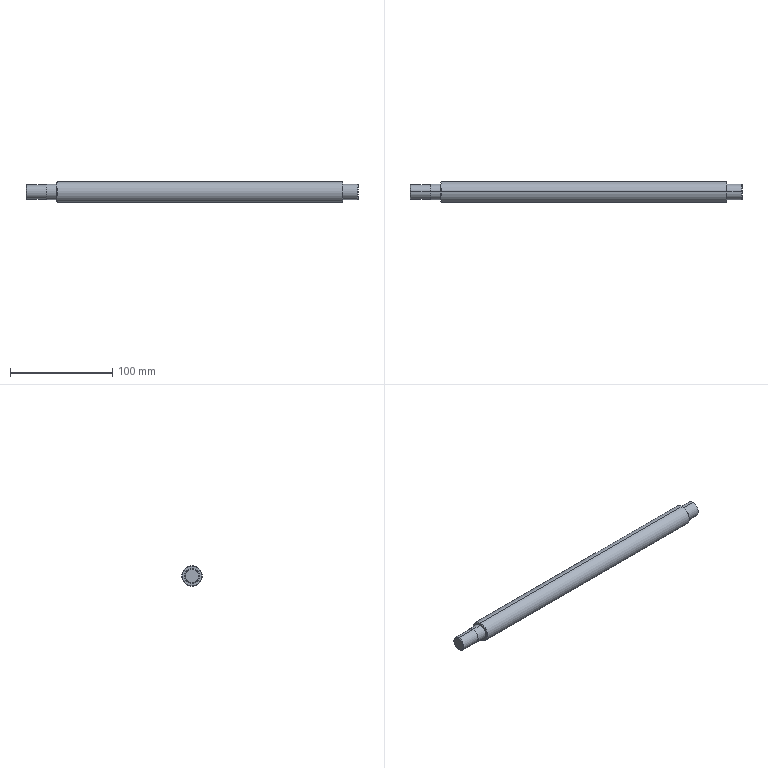Part | SolidWorks | features BaseBody 1 | 1 solid | 21 faces | box 325 x 20 x 20 mm | volume 95435 mm3 | cone 8 | cylinder 8 | plane 5 | commonest cylinder face diameters 15 x4 14 x2 20 x2
STEP:
#1=CARTESIAN_POINT('',(162.5,0.,7.));
#2=VERTEX_POINT('',#1);
#3=CARTESIAN_POINT('',(162.5,0.,-7.));
#4=VERTEX_POINT('',#3);
#5=CARTESIAN_POINT('',(162.5,0.,0.));
#6=DIRECTION('',(-1.,0.,0.));
#7=DIRECTION('',(0.,0.,1.));
#8=AXIS2_PLACEMENT_3D('',#5,#6,#7);
#9=CIRCLE('',#8,7.);
#10=EDGE_CURVE('',#2,#4,#9,.T.);
#11=ORIENTED_EDGE('',*,*,#10,.T.);
#12=CARTESIAN_POINT('',(162.,0.,-7.5));
#13=VERTEX_POINT('',#12);
#14=CARTESIAN_POINT('',(162.5,0.,-7.));
#15=DIRECTION('',(-0.7071,0.,-0.7071));
#16=VECTOR('',#15,1000.);
#17=LINE('',#14,#16);
#18=EDGE_CURVE('',#4,#13,#17,.T.);
#19=ORIENTED_EDGE('',*,*,#18,.T.);
#20=CARTESIAN_POINT('',(162.,0.,7.5));
#21=VERTEX_POINT('',#20);
#22=CARTESIAN_POINT('',(162.,0.,0.));
#23=DIRECTION('',(-1.,0.,0.));
#24=DIRECTION('',(0.,0.,1.));
#25=AXIS2_PLACEMENT_3D('',#22,#23,#24);
#26=CIRCLE('',#25,7.5);
#27=EDGE_CURVE('',#21,#13,#26,.T.);
#28=ORIENTED_EDGE('',*,*,#27,.F.);
#29=CARTESIAN_POINT('',(162.5,0.,7.));
#30=DIRECTION('',(-0.7071,0.,0.7071));
#31=VECTOR('',#30,1000.);
#32=LINE('',#29,#31);
#33=EDGE_CURVE('',#2,#21,#32,.T.);
#34=ORIENTED_EDGE('',*,*,#33,.F.);
#35=EDGE_LOOP('',(#11,#19,#28,#34));
#36=FACE_OUTER_BOUND('',#35,.T.);
#37=CARTESIAN_POINT('',(162.5,0.,0.));
#38=DIRECTION('',(-1.,0.,0.));
#39=DIRECTION('',(0.,0.,1.));
#40=AXIS2_PLACEMENT_3D('',#37,#38,#39);
#41=CONICAL_SURFACE('',#40,7.,0.7854);
#42=ADVANCED_FACE('',(#36),#41,.T.);
#43=ORIENTED_EDGE('',*,*,#27,.T.);
#44=CARTESIAN_POINT('',(147.5,0.,-7.5));
#45=VERTEX_POINT('',#44);
#46=CARTESIAN_POINT('',(-162.5,0.,-7.5));
#47=DIRECTION('',(-1.,0.,0.));
#48=VECTOR('',#47,1000.);
#49=LINE('',#46,#48);
#50=EDGE_CURVE('',#13,#45,#49,.T.);
#51=ORIENTED_EDGE('',*,*,#50,.T.);
#52=CARTESIAN_POINT('',(147.5,0.,7.5));
#53=VERTEX_POINT('',#52);
#54=CARTESIAN_POINT('',(147.5,0.,0.));
#55=DIRECTION('',(-1.,0.,0.));
#56=DIRECTION('',(0.,0.,1.));
#57=AXIS2_PLACEMENT_3D('',#54,#55,#56);
#58=CIRCLE('',#57,7.5);
#59=EDGE_CURVE('',#53,#45,#58,.T.);
#60=ORIENTED_EDGE('',*,*,#59,.F.);
#61=CARTESIAN_POINT('',(-162.5,0.,7.5));
#62=DIRECTION('',(-1.,0.,0.));
#63=VECTOR('',#62,1000.);
#64=LINE('',#61,#63);
#65=EDGE_CURVE('',#21,#53,#64,.T.);
#66=ORIENTED_EDGE('',*,*,#65,.F.);
#67=EDGE_LOOP('',(#43,#51,#60,#66));
#68=FACE_OUTER_BOUND('',#67,.T.);
#69=CARTESIAN_POINT('',(-162.5,0.,0.));
#70=DIRECTION('',(-1.,0.,0.));
#71=DIRECTION('',(0.,0.,1.));
#72=AXIS2_PLACEMENT_3D('',#69,#70,#71);
#73=CYLINDRICAL_SURFACE('',#72,7.5);
#74=ADVANCED_FACE('',(#68),#73,.T.);
#75=CARTESIAN_POINT('',(147.5,0.,9.5));
#76=VERTEX_POINT('',#75);
#77=CARTESIAN_POINT('',(147.5,0.,-9.5));
#78=VERTEX_POINT('',#77);
#79=CARTESIAN_POINT('',(147.5,0.,0.));
#80=DIRECTION('',(-1.,0.,0.));
#81=DIRECTION('',(0.,0.,1.));
#82=AXIS2_PLACEMENT_3D('',#79,#80,#81);
#83=CIRCLE('',#82,9.5);
#84=EDGE_CURVE('',#76,#78,#83,.T.);
#85=ORIENTED_EDGE('',*,*,#84,.T.);
#86=CARTESIAN_POINT('',(147.,0.,-10.));
#87=VERTEX_POINT('',#86);
#88=CARTESIAN_POINT('',(147.5,0.,-9.5));
#89=DIRECTION('',(-0.7071,0.,-0.7071));
#90=VECTOR('',#89,1000.);
#91=LINE('',#88,#90);
#92=EDGE_CURVE('',#78,#87,#91,.T.);
#93=ORIENTED_EDGE('',*,*,#92,.T.);
#94=CARTESIAN_POINT('',(147.,0.,10.));
#95=VERTEX_POINT('',#94);
#96=CARTESIAN_POINT('',(147.,0.,0.));
#97=DIRECTION('',(-1.,0.,0.));
#98=DIRECTION('',(0.,0.,1.));
#99=AXIS2_PLACEMENT_3D('',#96,#97,#98);
#100=CIRCLE('',#99,10.);
#101=EDGE_CURVE('',#95,#87,#100,.T.);
#102=ORIENTED_EDGE('',*,*,#101,.F.);
#103=CARTESIAN_POINT('',(147.5,0.,9.5));
#104=DIRECTION('',(-0.7071,0.,0.7071));
#105=VECTOR('',#104,1000.);
#106=LINE('',#103,#105);
#107=EDGE_CURVE('',#76,#95,#106,.T.);
#108=ORIENTED_EDGE('',*,*,#107,.F.);
#109=EDGE_LOOP('',(#85,#93,#102,#108));
#110=FACE_OUTER_BOUND('',#109,.T.);
#111=CARTESIAN_POINT('',(147.5,0.,0.));
#112=DIRECTION('',(-1.,0.,0.));
#113=DIRECTION('',(0.,0.,1.));
#114=AXIS2_PLACEMENT_3D('',#111,#112,#113);
#115=CONICAL_SURFACE('',#114,9.5,0.7854);
#116=ADVANCED_FACE('',(#110),#115,.T.);
#117=ORIENTED_EDGE('',*,*,#101,.T.);
#118=CARTESIAN_POINT('',(-132.,0.,-10.));
#119=VERTEX_POINT('',#118);
#120=CARTESIAN_POINT('',(-162.5,0.,-10.));
#121=DIRECTION('',(-1.,0.,0.));
#122=VECTOR('',#121,1000.);
#123=LINE('',#120,#122);
#124=EDGE_CURVE('',#87,#119,#123,.T.);
#125=ORIENTED_EDGE('',*,*,#124,.T.);
#126=CARTESIAN_POINT('',(-132.,0.,10.));
#127=VERTEX_POINT('',#126);
#128=CARTESIAN_POINT('',(-132.,0.,0.));
#129=DIRECTION('',(-1.,0.,0.));
#130=DIRECTION('',(0.,0.,1.));
#131=AXIS2_PLACEMENT_3D('',#128,#129,#130);
#132=CIRCLE('',#131,10.);
#133=EDGE_CURVE('',#127,#119,#132,.T.);
#134=ORIENTED_EDGE('',*,*,#133,.F.);
#135=CARTESIAN_POINT('',(-162.5,0.,10.));
#136=DIRECTION('',(-1.,0.,0.));
#137=VECTOR('',#136,1000.);
#138=LINE('',#135,#137);
#139=EDGE_CURVE('',#95,#127,#138,.T.);
#140=ORIENTED_EDGE('',*,*,#139,.F.);
#141=EDGE_LOOP('',(#117,#125,#134,#140));
#142=FACE_OUTER_BOUND('',#141,.T.);
#143=CARTESIAN_POINT('',(-162.5,0.,0.));
#144=DIRECTION('',(-1.,0.,0.));
#145=DIRECTION('',(0.,0.,1.));
#146=AXIS2_PLACEMENT_3D('',#143,#144,#145);
#147=CYLINDRICAL_SURFACE('',#146,10.);
#148=ADVANCED_FACE('',(#142),#147,.T.);
#149=CARTESIAN_POINT('',(-132.5,0.,9.5));
#150=VERTEX_POINT('',#149);
#151=CARTESIAN_POINT('',(-132.5,0.,-9.5));
#152=VERTEX_POINT('',#151);
#153=CARTESIAN_POINT('',(-132.5,0.,0.));
#154=DIRECTION('',(-1.,0.,0.));
#155=DIRECTION('',(0.,0.,1.));
#156=AXIS2_PLACEMENT_3D('',#153,#154,#155);
#157=CIRCLE('',#156,9.5);
#158=EDGE_CURVE('',#150,#152,#157,.T.);
#159=ORIENTED_EDGE('',*,*,#158,.F.);
#160=CARTESIAN_POINT('',(-132.,0.,10.));
#161=DIRECTION('',(0.7071,0.,0.7071));
#162=VECTOR('',#161,1000.);
#163=LINE('',#160,#162);
#164=EDGE_CURVE('',#150,#127,#163,.T.);
#165=ORIENTED_EDGE('',*,*,#164,.T.);
#166=ORIENTED_EDGE('',*,*,#133,.T.);
#167=CARTESIAN_POINT('',(-132.,0.,-10.));
#168=DIRECTION('',(0.7071,0.,-0.7071));
#169=VECTOR('',#168,1000.);
#170=LINE('',#167,#169);
#171=EDGE_CURVE('',#152,#119,#170,.T.);
#172=ORIENTED_EDGE('',*,*,#171,.F.);
#173=EDGE_LOOP('',(#159,#165,#166,#172));
#174=FACE_OUTER_BOUND('',#173,.T.);
#175=CARTESIAN_POINT('',(-132.,0.,0.));
#176=DIRECTION('',(1.,0.,0.));
#177=DIRECTION('',(0.,0.,-1.));
#178=AXIS2_PLACEMENT_3D('',#175,#176,#177);
#179=CONICAL_SURFACE('',#178,10.,0.7854);
#180=ADVANCED_FACE('',(#174),#179,.T.);
#181=CARTESIAN_POINT('',(-132.5,0.,7.5));
#182=VERTEX_POINT('',#181);
#183=CARTESIAN_POINT('',(-132.5,0.,-7.5));
#184=VERTEX_POINT('',#183);
#185=CARTESIAN_POINT('',(-132.5,0.,0.));
#186=DIRECTION('',(-1.,0.,0.));
#187=DIRECTION('',(0.,0.,1.));
#188=AXIS2_PLACEMENT_3D('',#185,#186,#187);
#189=CIRCLE('',#188,7.5);
#190=EDGE_CURVE('',#182,#184,#189,.T.);
#191=ORIENTED_EDGE('',*,*,#190,.T.);
#192=CARTESIAN_POINT('',(-142.5,0.,-7.5));
#193=VERTEX_POINT('',#192);
#194=CARTESIAN_POINT('',(-162.5,0.,-7.5));
#195=DIRECTION('',(-1.,0.,0.));
#196=VECTOR('',#195,1000.);
#197=LINE('',#194,#196);
#198=EDGE_CURVE('',#184,#193,#197,.T.);
#199=ORIENTED_EDGE('',*,*,#198,.T.);
#200=CARTESIAN_POINT('',(-142.5,0.,7.5));
#201=VERTEX_POINT('',#200);
#202=CARTESIAN_POINT('',(-142.5,0.,0.));
#203=DIRECTION('',(-1.,0.,0.));
#204=DIRECTION('',(0.,0.,1.));
#205=AXIS2_PLACEMENT_3D('',#202,#203,#204);
#206=CIRCLE('',#205,7.5);
#207=EDGE_CURVE('',#201,#193,#206,.T.);
#208=ORIENTED_EDGE('',*,*,#207,.F.);
#209=CARTESIAN_POINT('',(-162.5,0.,7.5));
#210=DIRECTION('',(-1.,0.,0.));
#211=VECTOR('',#210,1000.);
#212=LINE('',#209,#211);
#213=EDGE_CURVE('',#182,#201,#212,.T.);
#214=ORIENTED_EDGE('',*,*,#213,.F.);
#215=EDGE_LOOP('',(#191,#199,#208,#214));
#216=FACE_OUTER_BOUND('',#215,.T.);
#217=CARTESIAN_POINT('',(-162.5,0.,0.));
#218=DIRECTION('',(-1.,0.,0.));
#219=DIRECTION('',(0.,0.,1.));
#220=AXIS2_PLACEMENT_3D('',#217,#218,#219);
#221=CYLINDRICAL_SURFACE('',#220,7.5);
#222=ADVANCED_FACE('',(#216),#221,.T.);
#223=CARTESIAN_POINT('',(-142.5,0.,7.));
#224=VERTEX_POINT('',#223);
#225=CARTESIAN_POINT('',(-142.5,0.,-7.));
#226=VERTEX_POINT('',#225);
#227=CARTESIAN_POINT('',(-142.5,0.,0.));
#228=DIRECTION('',(-1.,0.,0.));
#229=DIRECTION('',(0.,0.,1.));
#230=AXIS2_PLACEMENT_3D('',#227,#228,#229);
#231=CIRCLE('',#230,7.);
#232=EDGE_CURVE('',#224,#226,#231,.T.);
#233=ORIENTED_EDGE('',*,*,#232,.T.);
#234=CARTESIAN_POINT('',(-162.,0.,-7.));
#235=VERTEX_POINT('',#234);
#236=CARTESIAN_POINT('',(-162.5,0.,-7.));
#237=DIRECTION('',(-1.,0.,0.));
#238=VECTOR('',#237,1000.);
#239=LINE('',#236,#238);
#240=EDGE_CURVE('',#226,#235,#239,.T.);
#241=ORIENTED_EDGE('',*,*,#240,.T.);
#242=CARTESIAN_POINT('',(-162.,0.,7.));
#243=VERTEX_POINT('',#242);
#244=CARTESIAN_POINT('',(-162.,0.,0.));
#245=DIRECTION('',(-1.,0.,0.));
#246=DIRECTION('',(0.,0.,1.));
#247=AXIS2_PLACEMENT_3D('',#244,#245,#246);
#248=CIRCLE('',#247,7.);
#249=EDGE_CURVE('',#243,#235,#248,.T.);
#250=ORIENTED_EDGE('',*,*,#249,.F.);
#251=CARTESIAN_POINT('',(-162.5,0.,7.));
#252=DIRECTION('',(-1.,0.,0.));
#253=VECTOR('',#252,1000.);
#254=LINE('',#251,#253);
#255=EDGE_CURVE('',#224,#243,#254,.T.);
#256=ORIENTED_EDGE('',*,*,#255,.F.);
#257=EDGE_LOOP('',(#233,#241,#250,#256));
#258=FACE_OUTER_BOUND('',#257,.T.);
#259=CARTESIAN_POINT('',(-162.5,0.,0.));
#260=DIRECTION('',(-1.,0.,0.));
#261=DIRECTION('',(0.,0.,1.));
#262=AXIS2_PLACEMENT_3D('',#259,#260,#261);
#263=CYLINDRICAL_SURFACE('',#262,7.);
#264=ADVANCED_FACE('',(#258),#263,.T.);
#265=CARTESIAN_POINT('',(-162.5,0.,6.5));
#266=VERTEX_POINT('',#265);
#267=CARTESIAN_POINT('',(-162.5,0.,-6.5));
#268=VERTEX_POINT('',#267);
#269=CARTESIAN_POINT('',(-162.5,0.,0.));
#270=DIRECTION('',(-1.,0.,0.));
#271=DIRECTION('',(0.,0.,1.));
#272=AXIS2_PLACEMENT_3D('',#269,#270,#271);
#273=CIRCLE('',#272,6.5);
#274=EDGE_CURVE('',#266,#268,#273,.T.);
#275=ORIENTED_EDGE('',*,*,#274,.F.);
#276=CARTESIAN_POINT('',(-162.,0.,7.));
#277=DIRECTION('',(0.7071,0.,0.7071));
#278=VECTOR('',#277,1000.);
#279=LINE('',#276,#278);
#280=EDGE_CURVE('',#266,#243,#279,.T.);
#281=ORIENTED_EDGE('',*,*,#280,.T.);
#282=ORIENTED_EDGE('',*,*,#249,.T.);
#283=CARTESIAN_POINT('',(-162.,0.,-7.));
#284=DIRECTION('',(0.7071,0.,-0.7071));
#285=VECTOR('',#284,1000.);
#286=LINE('',#283,#285);
#287=EDGE_CURVE('',#268,#235,#286,.T.);
#288=ORIENTED_EDGE('',*,*,#287,.F.);
#289=EDGE_LOOP('',(#275,#281,#282,#288));
#290=FACE_OUTER_BOUND('',#289,.T.);
#291=CARTESIAN_POINT('',(-162.,0.,0.));
#292=DIRECTION('',(1.,0.,0.));
#293=DIRECTION('',(0.,0.,-1.));
#294=AXIS2_PLACEMENT_3D('',#291,#292,#293);
#295=CONICAL_SURFACE('',#294,7.,0.7854);
#296=ADVANCED_FACE('',(#290),#295,.T.);
#297=ORIENTED_EDGE('',*,*,#10,.F.);
#298=CARTESIAN_POINT('',(162.5,0.,0.));
#299=DIRECTION('',(-1.,0.,0.));
#300=DIRECTION('',(0.,0.,1.));
#301=AXIS2_PLACEMENT_3D('',#298,#299,#300);
#302=CIRCLE('',#301,7.);
#303=EDGE_CURVE('',#4,#2,#302,.T.);
#304=ORIENTED_EDGE('',*,*,#303,.F.);
#305=EDGE_LOOP('',(#297,#304));
#306=FACE_OUTER_BOUND('',#305,.T.);
#307=CARTESIAN_POINT('',(162.5,7.,0.));
#308=DIRECTION('',(-1.,0.,0.));
#309=DIRECTION('',(0.,0.,1.));
#310=AXIS2_PLACEMENT_3D('',#307,#308,#309);
#311=PLANE('',#310);
#312=ADVANCED_FACE('',(#306),#311,.F.);
#313=ORIENTED_EDGE('',*,*,#59,.T.);
#314=CARTESIAN_POINT('',(147.5,0.,0.));
#315=DIRECTION('',(-1.,0.,0.));
#316=DIRECTION('',(0.,0.,1.));
#317=AXIS2_PLACEMENT_3D('',#314,#315,#316);
#318=CIRCLE('',#317,7.5);
#319=EDGE_CURVE('',#45,#53,#318,.T.);
#320=ORIENTED_EDGE('',*,*,#319,.T.);
#321=EDGE_LOOP('',(#313,#320));
#322=FACE_BOUND('',#321,.T.);
#323=ORIENTED_EDGE('',*,*,#84,.F.);
#324=CARTESIAN_POINT('',(147.5,0.,0.));
#325=DIRECTION('',(-1.,0.,0.));
#326=DIRECTION('',(0.,0.,1.));
#327=AXIS2_PLACEMENT_3D('',#324,#325,#326);
#328=CIRCLE('',#327,9.5);
#329=EDGE_CURVE('',#78,#76,#328,.T.);
#330=ORIENTED_EDGE('',*,*,#329,.F.);
#331=EDGE_LOOP('',(#323,#330));
#332=FACE_OUTER_BOUND('',#331,.T.);
#333=CARTESIAN_POINT('',(147.5,9.5,0.));
#334=DIRECTION('',(-1.,0.,0.));
#335=DIRECTION('',(0.,0.,1.));
#336=AXIS2_PLACEMENT_3D('',#333,#334,#335);
#337=PLANE('',#336);
#338=ADVANCED_FACE('',(#322,#332),#337,.F.);
#339=ORIENTED_EDGE('',*,*,#190,.F.);
#340=CARTESIAN_POINT('',(-132.5,0.,0.));
#341=DIRECTION('',(-1.,0.,0.));
#342=DIRECTION('',(0.,0.,1.));
#343=AXIS2_PLACEMENT_3D('',#340,#341,#342);
#344=CIRCLE('',#343,7.5);
#345=EDGE_CURVE('',#184,#182,#344,.T.);
#346=ORIENTED_EDGE('',*,*,#345,.F.);
#347=EDGE_LOOP('',(#339,#346));
#348=FACE_BOUND('',#347,.T.);
#349=CARTESIAN_POINT('',(-132.5,0.,0.));
#350=DIRECTION('',(-1.,0.,0.));
#351=DIRECTION('',(0.,0.,1.));
#352=AXIS2_PLACEMENT_3D('',#349,#350,#351);
#353=CIRCLE('',#352,9.5);
#354=EDGE_CURVE('',#152,#150,#353,.T.);
#355=ORIENTED_EDGE('',*,*,#354,.T.);
#356=ORIENTED_EDGE('',*,*,#158,.T.);
#357=EDGE_LOOP('',(#355,#356));
#358=FACE_OUTER_BOUND('',#357,.T.);
#359=CARTESIAN_POINT('',(-132.5,7.5,0.));
#360=DIRECTION('',(1.,0.,0.));
#361=DIRECTION('',(0.,1.,0.));
#362=AXIS2_PLACEMENT_3D('',#359,#360,#361);
#363=PLANE('',#362);
#364=ADVANCED_FACE('',(#348,#358),#363,.F.);
#365=ORIENTED_EDGE('',*,*,#232,.F.);
#366=CARTESIAN_POINT('',(-142.5,0.,0.));
#367=DIRECTION('',(-1.,0.,0.));
#368=DIRECTION('',(0.,0.,1.));
#369=AXIS2_PLACEMENT_3D('',#366,#367,#368);
#370=CIRCLE('',#369,7.);
#371=EDGE_CURVE('',#226,#224,#370,.T.);
#372=ORIENTED_EDGE('',*,*,#371,.F.);
#373=EDGE_LOOP('',(#365,#372));
#374=FACE_BOUND('',#373,.T.);
#375=ORIENTED_EDGE('',*,*,#207,.T.);
#376=CARTESIAN_POINT('',(-142.5,0.,0.));
#377=DIRECTION('',(-1.,0.,0.));
#378=DIRECTION('',(0.,0.,1.));
#379=AXIS2_PLACEMENT_3D('',#376,#377,#378);
#380=CIRCLE('',#379,7.5);
#381=EDGE_CURVE('',#193,#201,#380,.T.);
#382=ORIENTED_EDGE('',*,*,#381,.T.);
#383=EDGE_LOOP('',(#375,#382));
#384=FACE_OUTER_BOUND('',#383,.T.);
#385=CARTESIAN_POINT('',(-142.5,7.,0.));
#386=DIRECTION('',(1.,0.,0.));
#387=DIRECTION('',(0.,1.,0.));
#388=AXIS2_PLACEMENT_3D('',#385,#386,#387);
#389=PLANE('',#388);
#390=ADVANCED_FACE('',(#374,#384),#389,.F.);
#391=CARTESIAN_POINT('',(-162.5,0.,0.));
#392=DIRECTION('',(-1.,0.,0.));
#393=DIRECTION('',(0.,0.,1.));
#394=AXIS2_PLACEMENT_3D('',#391,#392,#393);
#395=CIRCLE('',#394,6.5);
#396=EDGE_CURVE('',#268,#266,#395,.T.);
#397=ORIENTED_EDGE('',*,*,#396,.T.);
#398=ORIENTED_EDGE('',*,*,#274,.T.);
#399=EDGE_LOOP('',(#397,#398));
#400=FACE_OUTER_BOUND('',#399,.T.);
#401=CARTESIAN_POINT('',(-162.5,0.,0.));
#402=DIRECTION('',(1.,0.,0.));
#403=DIRECTION('',(0.,1.,0.));
#404=AXIS2_PLACEMENT_3D('',#401,#402,#403);
#405=PLANE('',#404);
#406=ADVANCED_FACE('',(#400),#405,.F.);
#407=ORIENTED_EDGE('',*,*,#280,.F.);
#408=ORIENTED_EDGE('',*,*,#396,.F.);
#409=ORIENTED_EDGE('',*,*,#287,.T.);
#410=CARTESIAN_POINT('',(-162.,0.,0.));
#411=DIRECTION('',(-1.,0.,0.));
#412=DIRECTION('',(0.,0.,1.));
#413=AXIS2_PLACEMENT_3D('',#410,#411,#412);
#414=CIRCLE('',#413,7.);
#415=EDGE_CURVE('',#235,#243,#414,.T.);
#416=ORIENTED_EDGE('',*,*,#415,.T.);
#417=EDGE_LOOP('',(#407,#408,#409,#416));
#418=FACE_OUTER_BOUND('',#417,.T.);
#419=CARTESIAN_POINT('',(-162.,0.,0.));
#420=DIRECTION('',(1.,0.,0.));
#421=DIRECTION('',(0.,0.,-1.));
#422=AXIS2_PLACEMENT_3D('',#419,#420,#421);
#423=CONICAL_SURFACE('',#422,7.,0.7854);
#424=ADVANCED_FACE('',(#418),#423,.T.);
#425=ORIENTED_EDGE('',*,*,#240,.F.);
#426=ORIENTED_EDGE('',*,*,#371,.T.);
#427=ORIENTED_EDGE('',*,*,#255,.T.);
#428=ORIENTED_EDGE('',*,*,#415,.F.);
#429=EDGE_LOOP('',(#425,#426,#427,#428));
#430=FACE_OUTER_BOUND('',#429,.T.);
#431=CARTESIAN_POINT('',(-162.5,0.,0.));
#432=DIRECTION('',(-1.,0.,0.));
#433=DIRECTION('',(0.,0.,1.));
#434=AXIS2_PLACEMENT_3D('',#431,#432,#433);
#435=CYLINDRICAL_SURFACE('',#434,7.);
#436=ADVANCED_FACE('',(#430),#435,.T.);
#437=ORIENTED_EDGE('',*,*,#198,.F.);
#438=ORIENTED_EDGE('',*,*,#345,.T.);
#439=ORIENTED_EDGE('',*,*,#213,.T.);
#440=ORIENTED_EDGE('',*,*,#381,.F.);
#441=EDGE_LOOP('',(#437,#438,#439,#440));
#442=FACE_OUTER_BOUND('',#441,.T.);
#443=CARTESIAN_POINT('',(-162.5,0.,0.));
#444=DIRECTION('',(-1.,0.,0.));
#445=DIRECTION('',(0.,0.,1.));
#446=AXIS2_PLACEMENT_3D('',#443,#444,#445);
#447=CYLINDRICAL_SURFACE('',#446,7.5);
#448=ADVANCED_FACE('',(#442),#447,.T.);
#449=ORIENTED_EDGE('',*,*,#164,.F.);
#450=ORIENTED_EDGE('',*,*,#354,.F.);
#451=ORIENTED_EDGE('',*,*,#171,.T.);
#452=CARTESIAN_POINT('',(-132.,0.,0.));
#453=DIRECTION('',(-1.,0.,0.));
#454=DIRECTION('',(0.,0.,1.));
#455=AXIS2_PLACEMENT_3D('',#452,#453,#454);
#456=CIRCLE('',#455,10.);
#457=EDGE_CURVE('',#119,#127,#456,.T.);
#458=ORIENTED_EDGE('',*,*,#457,.T.);
#459=EDGE_LOOP('',(#449,#450,#451,#458));
#460=FACE_OUTER_BOUND('',#459,.T.);
#461=CARTESIAN_POINT('',(-132.,0.,0.));
#462=DIRECTION('',(1.,0.,0.));
#463=DIRECTION('',(0.,0.,-1.));
#464=AXIS2_PLACEMENT_3D('',#461,#462,#463);
#465=CONICAL_SURFACE('',#464,10.,0.7854);
#466=ADVANCED_FACE('',(#460),#465,.T.);
#467=ORIENTED_EDGE('',*,*,#124,.F.);
#468=CARTESIAN_POINT('',(147.,0.,0.));
#469=DIRECTION('',(-1.,0.,0.));
#470=DIRECTION('',(0.,0.,1.));
#471=AXIS2_PLACEMENT_3D('',#468,#469,#470);
#472=CIRCLE('',#471,10.);
#473=EDGE_CURVE('',#87,#95,#472,.T.);
#474=ORIENTED_EDGE('',*,*,#473,.T.);
#475=ORIENTED_EDGE('',*,*,#139,.T.);
#476=ORIENTED_EDGE('',*,*,#457,.F.);
#477=EDGE_LOOP('',(#467,#474,#475,#476));
#478=FACE_OUTER_BOUND('',#477,.T.);
#479=CARTESIAN_POINT('',(-162.5,0.,0.));
#480=DIRECTION('',(-1.,0.,0.));
#481=DIRECTION('',(0.,0.,1.));
#482=AXIS2_PLACEMENT_3D('',#479,#480,#481);
#483=CYLINDRICAL_SURFACE('',#482,10.);
#484=ADVANCED_FACE('',(#478),#483,.T.);
#485=ORIENTED_EDGE('',*,*,#92,.F.);
#486=ORIENTED_EDGE('',*,*,#329,.T.);
#487=ORIENTED_EDGE('',*,*,#107,.T.);
#488=ORIENTED_EDGE('',*,*,#473,.F.);
#489=EDGE_LOOP('',(#485,#486,#487,#488));
#490=FACE_OUTER_BOUND('',#489,.T.);
#491=CARTESIAN_POINT('',(147.5,0.,0.));
#492=DIRECTION('',(-1.,0.,0.));
#493=DIRECTION('',(0.,0.,1.));
#494=AXIS2_PLACEMENT_3D('',#491,#492,#493);
#495=CONICAL_SURFACE('',#494,9.5,0.7854);
#496=ADVANCED_FACE('',(#490),#495,.T.);
#497=ORIENTED_EDGE('',*,*,#50,.F.);
#498=CARTESIAN_POINT('',(162.,0.,0.));
#499=DIRECTION('',(-1.,0.,0.));
#500=DIRECTION('',(0.,0.,1.));
#501=AXIS2_PLACEMENT_3D('',#498,#499,#500);
#502=CIRCLE('',#501,7.5);
#503=EDGE_CURVE('',#13,#21,#502,.T.);
#504=ORIENTED_EDGE('',*,*,#503,.T.);
#505=ORIENTED_EDGE('',*,*,#65,.T.);
#506=ORIENTED_EDGE('',*,*,#319,.F.);
#507=EDGE_LOOP('',(#497,#504,#505,#506));
#508=FACE_OUTER_BOUND('',#507,.T.);
#509=CARTESIAN_POINT('',(-162.5,0.,0.));
#510=DIRECTION('',(-1.,0.,0.));
#511=DIRECTION('',(0.,0.,1.));
#512=AXIS2_PLACEMENT_3D('',#509,#510,#511);
#513=CYLINDRICAL_SURFACE('',#512,7.5);
#514=ADVANCED_FACE('',(#508),#513,.T.);
#515=ORIENTED_EDGE('',*,*,#18,.F.);
#516=ORIENTED_EDGE('',*,*,#303,.T.);
#517=ORIENTED_EDGE('',*,*,#33,.T.);
#518=ORIENTED_EDGE('',*,*,#503,.F.);
#519=EDGE_LOOP('',(#515,#516,#517,#518));
#520=FACE_OUTER_BOUND('',#519,.T.);
#521=CARTESIAN_POINT('',(162.5,0.,0.));
#522=DIRECTION('',(-1.,0.,0.));
#523=DIRECTION('',(0.,0.,1.));
#524=AXIS2_PLACEMENT_3D('',#521,#522,#523);
#525=CONICAL_SURFACE('',#524,7.,0.7854);
#526=ADVANCED_FACE('',(#520),#525,.T.);
#527=CLOSED_SHELL('',(#42,#74,#116,#148,#180,#222,#264,#296,#312,#338,#364,#390,#406,#424,#436,#448,#466,#484,#496,#514,#526));
#528=MANIFOLD_SOLID_BREP('',#527);
#529=CARTESIAN_POINT('',(0.,0.,0.));
#530=DIRECTION('',(0.,0.,1.));
#531=DIRECTION('',(1.,0.,0.));
#532=AXIS2_PLACEMENT_3D('',#529,#530,#531);
#533=(LENGTH_UNIT()NAMED_UNIT(*)SI_UNIT(.MILLI.,.METRE.));
#534=UNCERTAINTY_MEASURE_WITH_UNIT(LENGTH_MEASURE(0.00001),#533,'','');
#535=(NAMED_UNIT(*)PLANE_ANGLE_UNIT()SI_UNIT($,.RADIAN.));
#536=(NAMED_UNIT(*)SI_UNIT($,.STERADIAN.)SOLID_ANGLE_UNIT());
#537=(GEOMETRIC_REPRESENTATION_CONTEXT(3)GLOBAL_UNCERTAINTY_ASSIGNED_CONTEXT((#534))GLOBAL_UNIT_ASSIGNED_CONTEXT((#533,#535,#536))REPRESENTATION_CONTEXT('',''));
#538=ADVANCED_BREP_SHAPE_REPRESENTATION('',(#528,#532),#537);